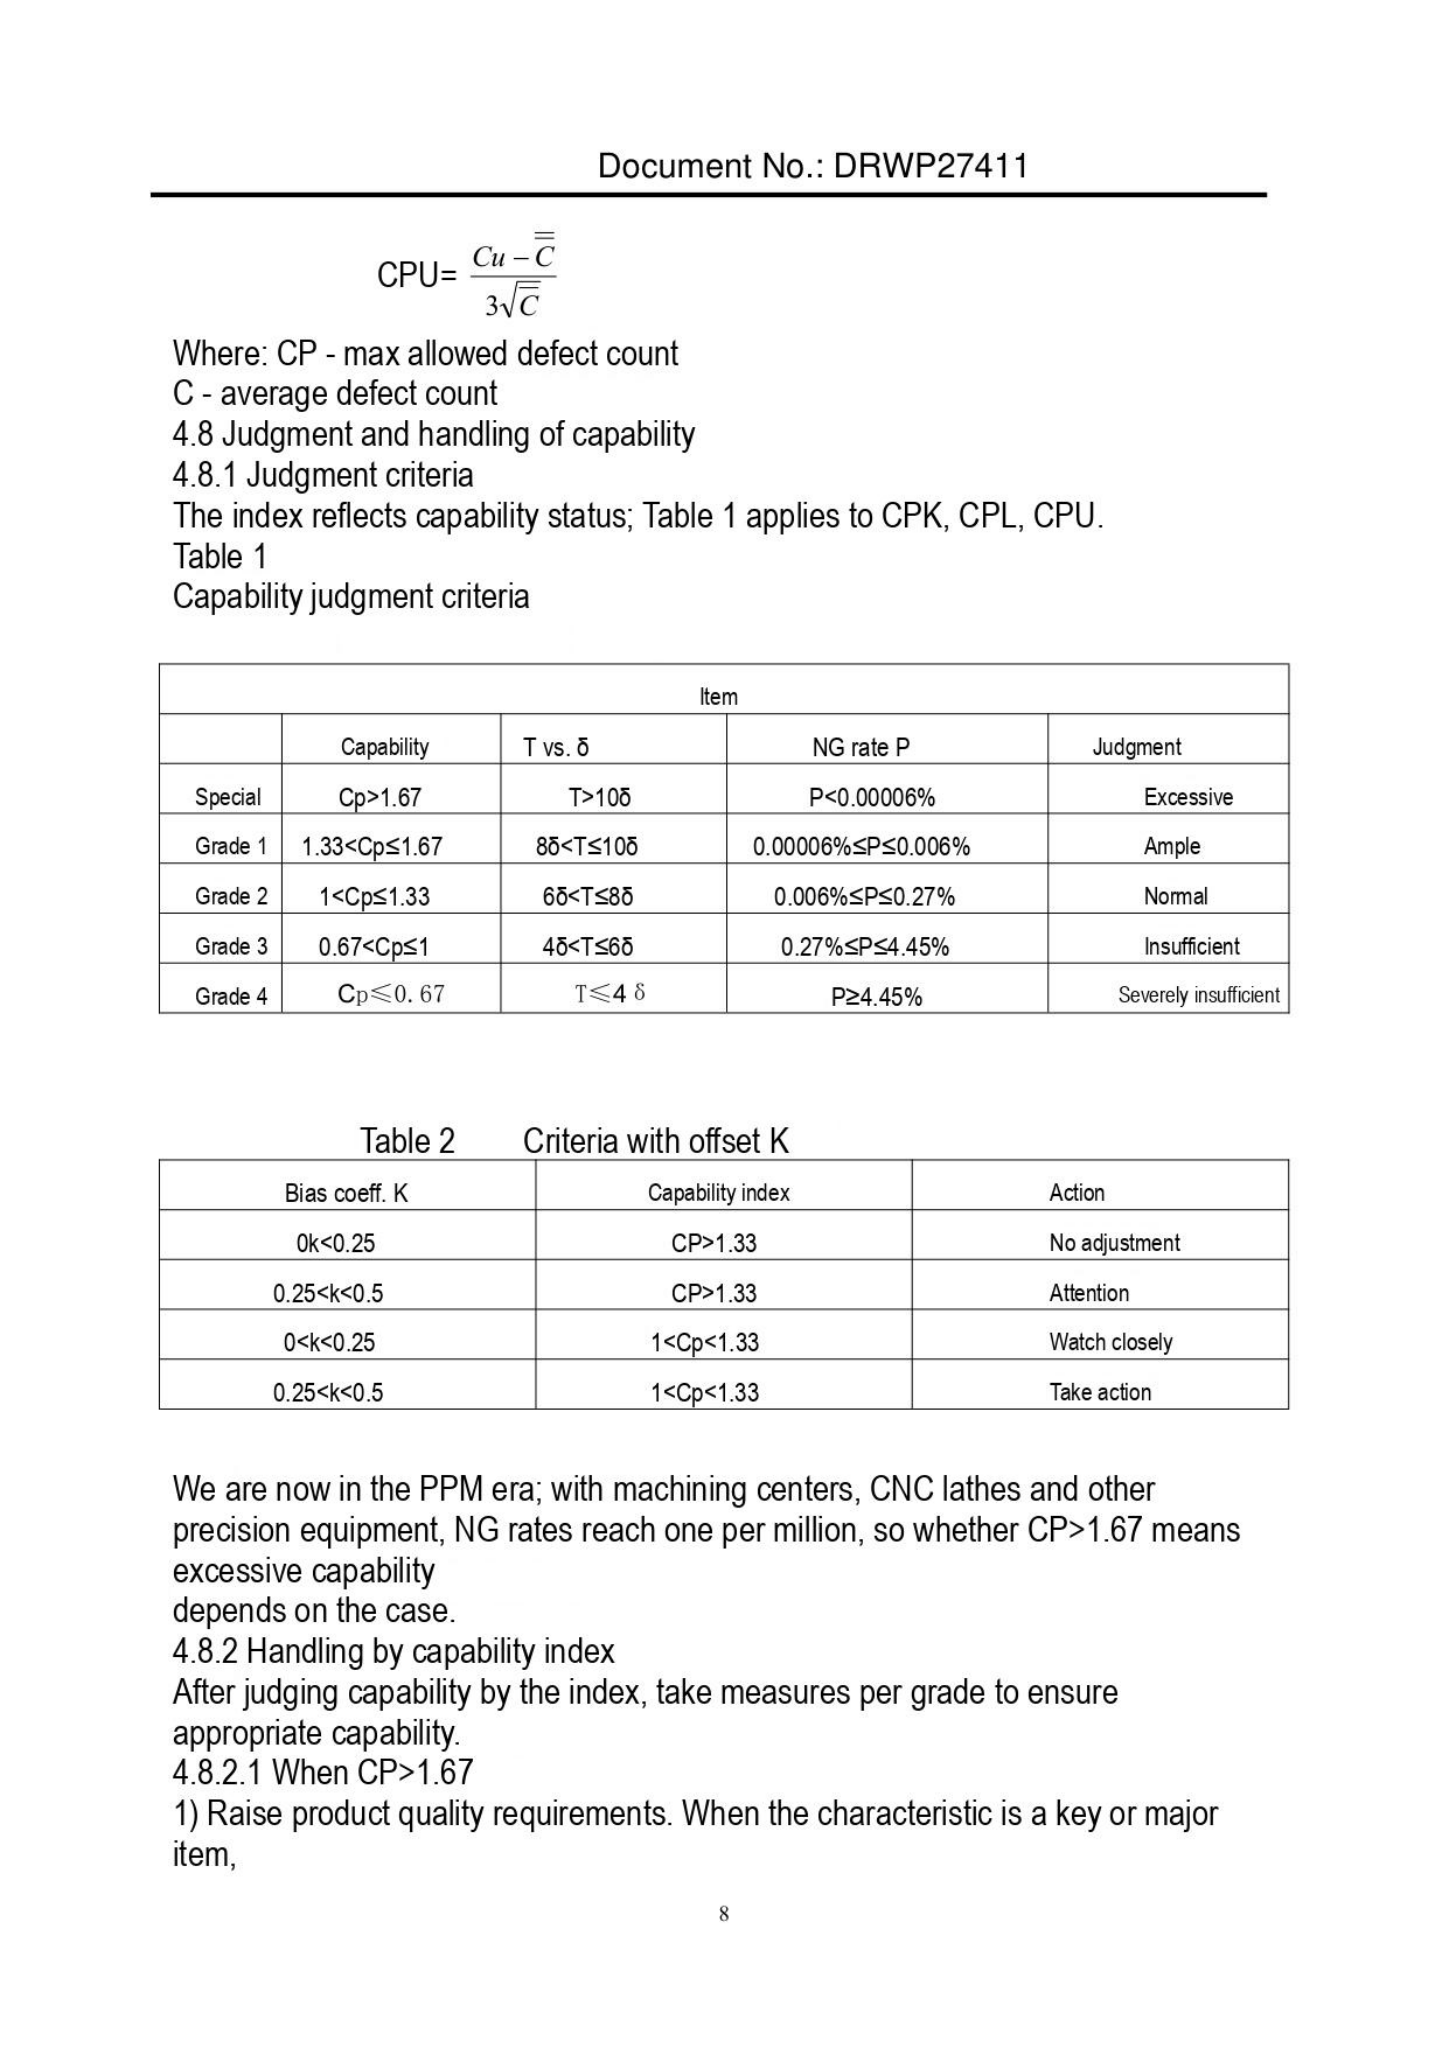Document No.: DRWP27411

CPU= (Cu − C̿) / (3√C̿)

Where: CP - max allowed defect count
C - average defect count
4.8 Judgment and handling of capability
4.8.1 Judgment criteria
The index reflects capability status; Table 1 applies to CPK, CPL, CPU.
Table 1
Capability judgment criteria

| Item | | | | |
|---|---|---|---|---|
| | Capability | T vs. δ | NG rate P | Judgment |
| Special | Cp>1.67 | T>10δ | P<0.00006% | Excessive |
| Grade 1 | 1.33<Cp≤1.67 | 8δ<T≤10δ | 0.00006%≤P≤0.006% | Ample |
| Grade 2 | 1<Cp≤1.33 | 6δ<T≤8δ | 0.006%≤P≤0.27% | Normal |
| Grade 3 | 0.67<Cp≤1 | 4δ<T≤6δ | 0.27%≤P≤4.45% | Insufficient |
| Grade 4 | Cp≤0. 67 | T≤4 δ | P≥4.45% | Severely insufficient |

Table 2 Criteria with offset K

| Bias coeff. K | Capability index | Action |
|---|---|---|
| 0k<0.25 | CP>1.33 | No adjustment |
| 0.25<k<0.5 | CP>1.33 | Attention |
| 0<k<0.25 | 1<Cp<1.33 | Watch closely |
| 0.25<k<0.5 | 1<Cp<1.33 | Take action |

We are now in the PPM era; with machining centers, CNC lathes and other precision equipment, NG rates reach one per million, so whether CP>1.67 means excessive capability
depends on the case.
4.8.2 Handling by capability index
After judging capability by the index, take measures per grade to ensure appropriate capability.
4.8.2.1 When CP>1.67
1) Raise product quality requirements. When the characteristic is a key or major item,

8
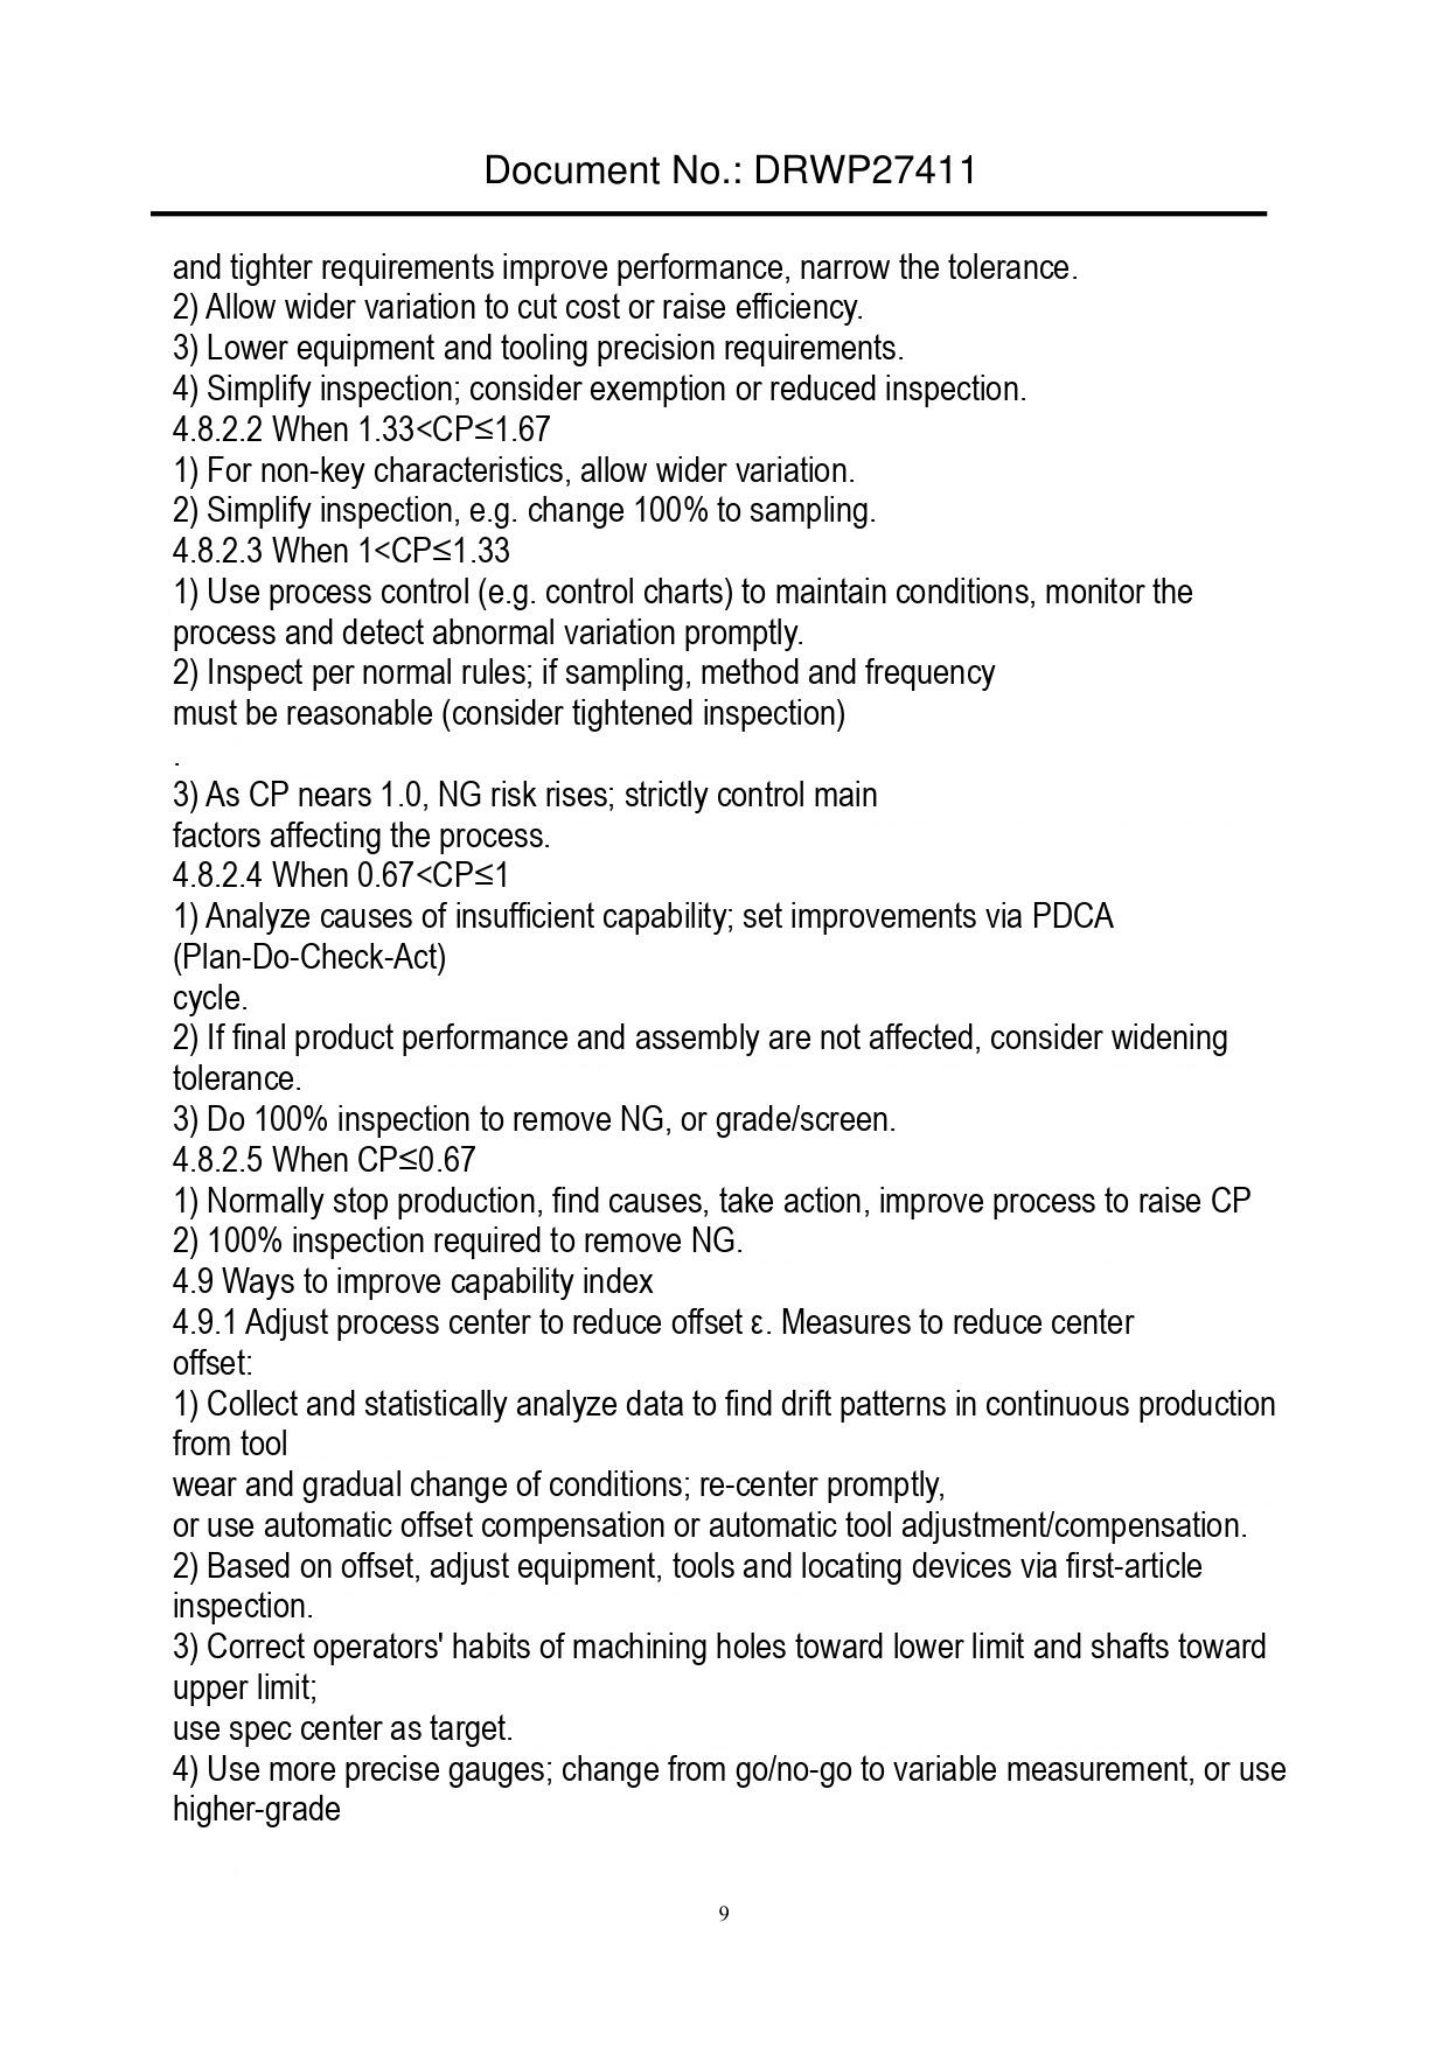Document No.: DRWP27411

and tighter requirements improve performance, narrow the tolerance.
2) Allow wider variation to cut cost or raise efficiency.
3) Lower equipment and tooling precision requirements.
4) Simplify inspection; consider exemption or reduced inspection.
4.8.2.2 When 1.33<CP≤1.67
1) For non-key characteristics, allow wider variation.
2) Simplify inspection, e.g. change 100% to sampling.
4.8.2.3 When 1<CP≤1.33
1) Use process control (e.g. control charts) to maintain conditions, monitor the process and detect abnormal variation promptly.
2) Inspect per normal rules; if sampling, method and frequency
must be reasonable (consider tightened inspection)
.
3) As CP nears 1.0, NG risk rises; strictly control main
factors affecting the process.
4.8.2.4 When 0.67<CP≤1
1) Analyze causes of insufficient capability; set improvements via PDCA
(Plan-Do-Check-Act)
cycle.
2) If final product performance and assembly are not affected, consider widening tolerance.
3) Do 100% inspection to remove NG, or grade/screen.
4.8.2.5 When CP≤0.67
1) Normally stop production, find causes, take action, improve process to raise CP
2) 100% inspection required to remove NG.
4.9 Ways to improve capability index
4.9.1 Adjust process center to reduce offset ε. Measures to reduce center
offset:
1) Collect and statistically analyze data to find drift patterns in continuous production from tool
wear and gradual change of conditions; re-center promptly,
or use automatic offset compensation or automatic tool adjustment/compensation.
2) Based on offset, adjust equipment, tools and locating devices via first-article inspection.
3) Correct operators' habits of machining holes toward lower limit and shafts toward upper limit;
use spec center as target.
4) Use more precise gauges; change from go/no-go to variable measurement, or use higher-grade

9
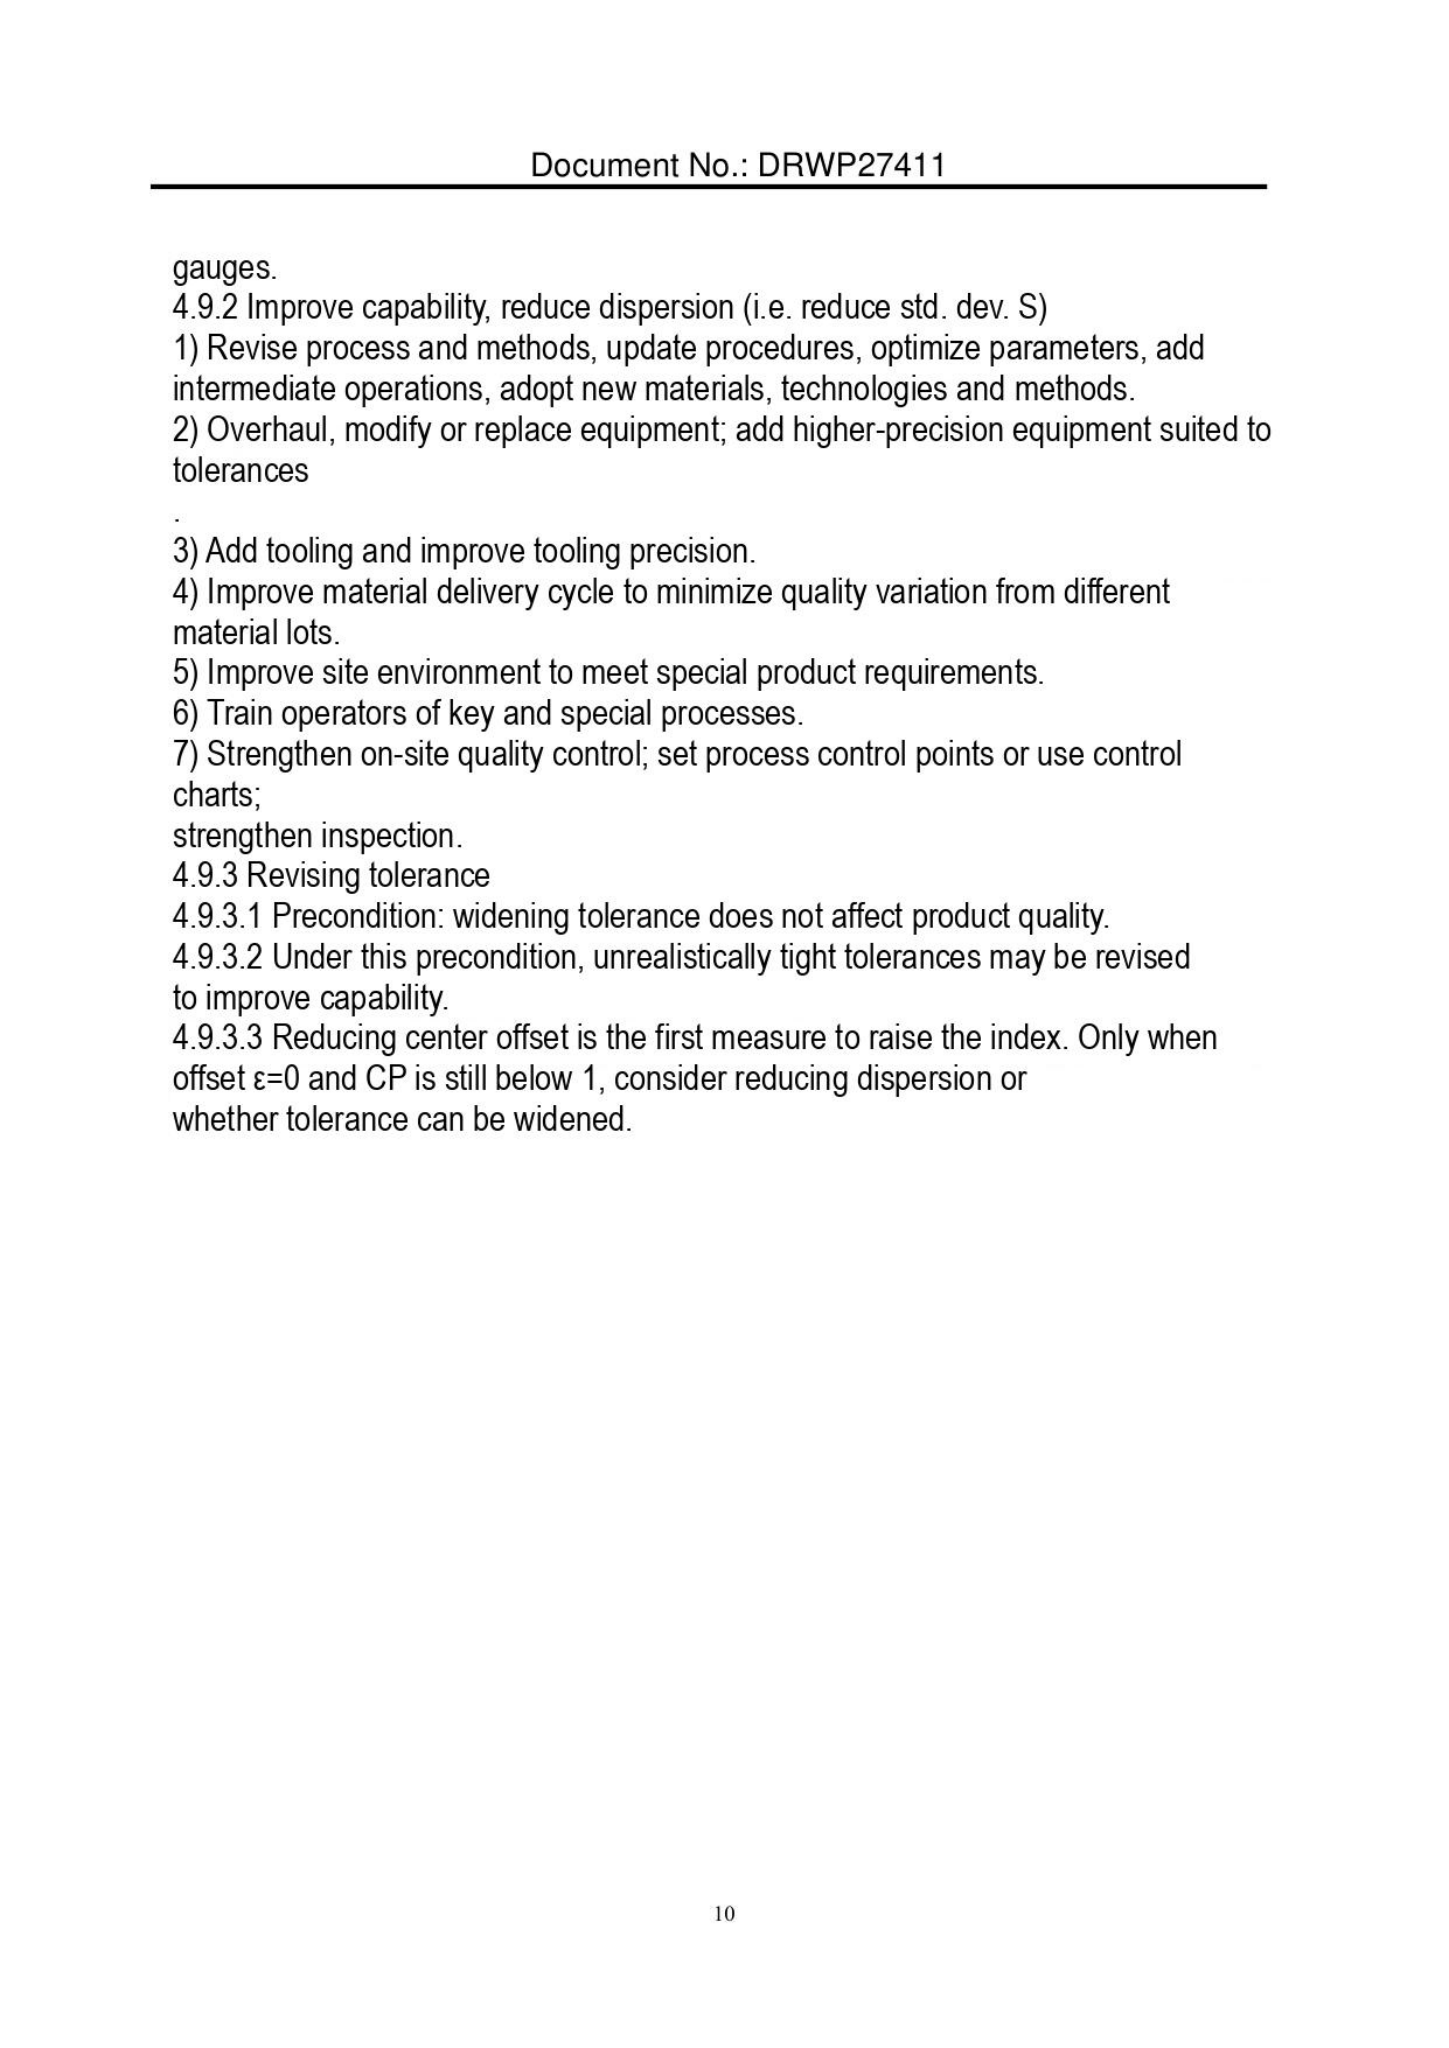Document No.: DRWP27411

gauges.
4.9.2 Improve capability, reduce dispersion (i.e. reduce std. dev. S)
1) Revise process and methods, update procedures, optimize parameters, add intermediate operations, adopt new materials, technologies and methods.
2) Overhaul, modify or replace equipment; add higher-precision equipment suited to tolerances
.
3) Add tooling and improve tooling precision.
4) Improve material delivery cycle to minimize quality variation from different material lots.
5) Improve site environment to meet special product requirements.
6) Train operators of key and special processes.
7) Strengthen on-site quality control; set process control points or use control charts;
strengthen inspection.
4.9.3 Revising tolerance
4.9.3.1 Precondition: widening tolerance does not affect product quality.
4.9.3.2 Under this precondition, unrealistically tight tolerances may be revised to improve capability.
4.9.3.3 Reducing center offset is the first measure to raise the index. Only when offset ε=0 and CP is still below 1, consider reducing dispersion or whether tolerance can be widened.

10